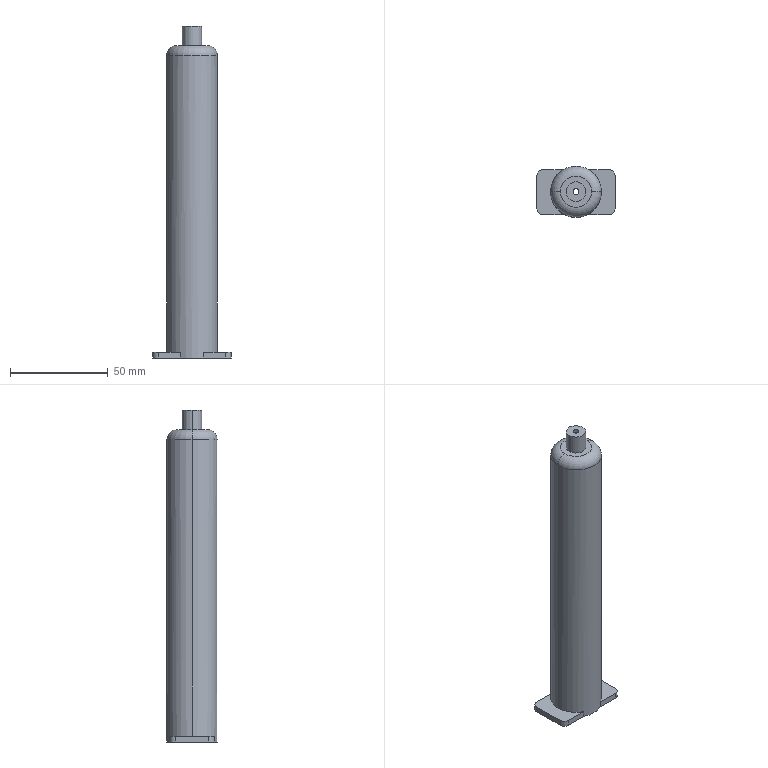Part | NX | features BREP 1 | 1 solid | 31 faces | box 40 x 26 x 170 mm | volume 26319 mm3 | cylinder 14 | plane 13 | torus 4 | commonest cylinder face diameters 6 x6 3 x2 10 x2 22 x2 26 x2
STEP:
#1=CARTESIAN_POINT('',(-1.5,0.,83.));
#2=VERTEX_POINT('',#1);
#3=CARTESIAN_POINT('',(1.5,0.,83.));
#4=VERTEX_POINT('',#3);
#5=CARTESIAN_POINT('',(0.,0.,83.));
#6=DIRECTION('',(0.,0.,1.));
#7=DIRECTION('',(1.,0.,0.));
#8=AXIS2_PLACEMENT_3D('',#5,#6,#7);
#9=CIRCLE('',#8,1.5);
#10=EDGE_CURVE('',#2,#4,#9,.T.);
#11=ORIENTED_EDGE('',*,*,#10,.F.);
#12=CARTESIAN_POINT('',(-1.5,0.,85.));
#13=VERTEX_POINT('',#12);
#14=CARTESIAN_POINT('',(-1.5,0.,75.));
#15=DIRECTION('',(0.,0.,1.));
#16=VECTOR('',#15,1000.);
#17=LINE('',#14,#16);
#18=EDGE_CURVE('',#13,#2,#17,.F.);
#19=ORIENTED_EDGE('',*,*,#18,.F.);
#20=CARTESIAN_POINT('',(1.5,0.,85.));
#21=VERTEX_POINT('',#20);
#22=CARTESIAN_POINT('',(0.,0.,85.));
#23=DIRECTION('',(0.,0.,1.));
#24=DIRECTION('',(1.,0.,0.));
#25=AXIS2_PLACEMENT_3D('',#22,#23,#24);
#26=CIRCLE('',#25,1.5);
#27=EDGE_CURVE('',#13,#21,#26,.T.);
#28=ORIENTED_EDGE('',*,*,#27,.T.);
#29=CARTESIAN_POINT('',(1.5,0.,75.));
#30=DIRECTION('',(0.,0.,1.));
#31=VECTOR('',#30,1000.);
#32=LINE('',#29,#31);
#33=EDGE_CURVE('',#21,#4,#32,.F.);
#34=ORIENTED_EDGE('',*,*,#33,.T.);
#35=EDGE_LOOP('',(#11,#19,#28,#34));
#36=FACE_BOUND('',#35,.T.);
#37=CARTESIAN_POINT('',(0.,0.,75.));
#38=DIRECTION('',(0.,0.,1.));
#39=DIRECTION('',(1.,0.,0.));
#40=AXIS2_PLACEMENT_3D('',#37,#38,#39);
#41=CYLINDRICAL_SURFACE('',#40,1.5);
#42=ADVANCED_FACE('',(#36),#41,.F.);
#43=CARTESIAN_POINT('',(11.,0.,70.));
#44=VERTEX_POINT('',#43);
#45=CARTESIAN_POINT('',(-11.,0.,70.));
#46=VERTEX_POINT('',#45);
#47=CARTESIAN_POINT('',(0.,0.,70.));
#48=DIRECTION('',(0.,0.,-1.));
#49=DIRECTION('',(-1.,0.,0.));
#50=AXIS2_PLACEMENT_3D('',#47,#48,#49);
#51=CIRCLE('',#50,11.);
#52=EDGE_CURVE('',#44,#46,#51,.T.);
#53=ORIENTED_EDGE('',*,*,#52,.T.);
#54=CARTESIAN_POINT('',(-8.,0.,73.));
#55=VERTEX_POINT('',#54);
#56=CARTESIAN_POINT('',(-8.,0.,70.));
#57=DIRECTION('',(0.,1.,0.));
#58=DIRECTION('',(-1.,0.,0.));
#59=AXIS2_PLACEMENT_3D('',#56,#57,#58);
#60=CIRCLE('',#59,3.);
#61=EDGE_CURVE('',#55,#46,#60,.F.);
#62=ORIENTED_EDGE('',*,*,#61,.F.);
#63=CARTESIAN_POINT('',(8.,0.,73.));
#64=VERTEX_POINT('',#63);
#65=CARTESIAN_POINT('',(0.,0.,73.));
#66=DIRECTION('',(0.,0.,1.));
#67=DIRECTION('',(1.,0.,0.));
#68=AXIS2_PLACEMENT_3D('',#65,#66,#67);
#69=CIRCLE('',#68,8.);
#70=EDGE_CURVE('',#55,#64,#69,.T.);
#71=ORIENTED_EDGE('',*,*,#70,.T.);
#72=CARTESIAN_POINT('',(8.,0.,70.));
#73=DIRECTION('',(0.,-1.,0.));
#74=DIRECTION('',(0.,0.,-1.));
#75=AXIS2_PLACEMENT_3D('',#72,#73,#74);
#76=CIRCLE('',#75,3.);
#77=EDGE_CURVE('',#64,#44,#76,.F.);
#78=ORIENTED_EDGE('',*,*,#77,.T.);
#79=EDGE_LOOP('',(#53,#62,#71,#78));
#80=FACE_BOUND('',#79,.T.);
#81=CARTESIAN_POINT('',(0.,0.,70.));
#82=DIRECTION('',(0.,0.,1.));
#83=DIRECTION('',(1.,0.,0.));
#84=AXIS2_PLACEMENT_3D('',#81,#82,#83);
#85=TOROIDAL_SURFACE('',#84,8.,3.);
#86=ADVANCED_FACE('',(#80),#85,.F.);
#87=CARTESIAN_POINT('',(-3.,0.,73.));
#88=VERTEX_POINT('',#87);
#89=CARTESIAN_POINT('',(3.,0.,73.));
#90=VERTEX_POINT('',#89);
#91=CARTESIAN_POINT('',(0.,0.,73.));
#92=DIRECTION('',(0.,0.,1.));
#93=DIRECTION('',(1.,0.,0.));
#94=AXIS2_PLACEMENT_3D('',#91,#92,#93);
#95=CIRCLE('',#94,3.);
#96=EDGE_CURVE('',#88,#90,#95,.T.);
#97=ORIENTED_EDGE('',*,*,#96,.F.);
#98=CARTESIAN_POINT('',(-3.,0.,83.));
#99=VERTEX_POINT('',#98);
#100=CARTESIAN_POINT('',(-3.,0.,75.));
#101=DIRECTION('',(0.,0.,1.));
#102=VECTOR('',#101,1000.);
#103=LINE('',#100,#102);
#104=EDGE_CURVE('',#99,#88,#103,.F.);
#105=ORIENTED_EDGE('',*,*,#104,.F.);
#106=CARTESIAN_POINT('',(3.,0.,83.));
#107=VERTEX_POINT('',#106);
#108=CARTESIAN_POINT('',(0.,0.,83.));
#109=DIRECTION('',(0.,0.,1.));
#110=DIRECTION('',(1.,0.,0.));
#111=AXIS2_PLACEMENT_3D('',#108,#109,#110);
#112=CIRCLE('',#111,3.);
#113=EDGE_CURVE('',#99,#107,#112,.T.);
#114=ORIENTED_EDGE('',*,*,#113,.T.);
#115=CARTESIAN_POINT('',(3.,0.,75.));
#116=DIRECTION('',(0.,0.,1.));
#117=VECTOR('',#116,1000.);
#118=LINE('',#115,#117);
#119=EDGE_CURVE('',#107,#90,#118,.F.);
#120=ORIENTED_EDGE('',*,*,#119,.T.);
#121=EDGE_LOOP('',(#97,#105,#114,#120));
#122=FACE_BOUND('',#121,.T.);
#123=CARTESIAN_POINT('',(0.,0.,75.));
#124=DIRECTION('',(0.,0.,1.));
#125=DIRECTION('',(1.,0.,0.));
#126=AXIS2_PLACEMENT_3D('',#123,#124,#125);
#127=CYLINDRICAL_SURFACE('',#126,3.);
#128=ADVANCED_FACE('',(#122),#127,.F.);
#129=ORIENTED_EDGE('',*,*,#52,.F.);
#130=CARTESIAN_POINT('',(11.,0.,-85.));
#131=VERTEX_POINT('',#130);
#132=CARTESIAN_POINT('',(11.,0.,85.));
#133=DIRECTION('',(0.,0.,-1.));
#134=VECTOR('',#133,1000.);
#135=LINE('',#132,#134);
#136=EDGE_CURVE('',#44,#131,#135,.T.);
#137=ORIENTED_EDGE('',*,*,#136,.T.);
#138=CARTESIAN_POINT('',(-11.,0.,-85.));
#139=VERTEX_POINT('',#138);
#140=CARTESIAN_POINT('',(0.,0.,-85.));
#141=DIRECTION('',(0.,0.,1.));
#142=DIRECTION('',(1.,0.,0.));
#143=AXIS2_PLACEMENT_3D('',#140,#141,#142);
#144=CIRCLE('',#143,11.);
#145=EDGE_CURVE('',#139,#131,#144,.T.);
#146=ORIENTED_EDGE('',*,*,#145,.F.);
#147=CARTESIAN_POINT('',(-11.,0.,85.));
#148=DIRECTION('',(0.,0.,-1.));
#149=VECTOR('',#148,1000.);
#150=LINE('',#147,#149);
#151=EDGE_CURVE('',#46,#139,#150,.T.);
#152=ORIENTED_EDGE('',*,*,#151,.F.);
#153=EDGE_LOOP('',(#129,#137,#146,#152));
#154=FACE_BOUND('',#153,.T.);
#155=CARTESIAN_POINT('',(0.,0.,85.));
#156=DIRECTION('',(0.,0.,-1.));
#157=DIRECTION('',(-1.,0.,0.));
#158=AXIS2_PLACEMENT_3D('',#155,#156,#157);
#159=CYLINDRICAL_SURFACE('',#158,11.);
#160=ADVANCED_FACE('',(#154),#159,.F.);
#161=CARTESIAN_POINT('',(-13.,0.,70.));
#162=VERTEX_POINT('',#161);
#163=CARTESIAN_POINT('',(13.,0.,70.));
#164=VERTEX_POINT('',#163);
#165=CARTESIAN_POINT('',(0.,0.,70.));
#166=DIRECTION('',(0.,0.,-1.));
#167=DIRECTION('',(1.,0.,0.));
#168=AXIS2_PLACEMENT_3D('',#165,#166,#167);
#169=CIRCLE('',#168,13.);
#170=EDGE_CURVE('',#162,#164,#169,.T.);
#171=ORIENTED_EDGE('',*,*,#170,.F.);
#172=CARTESIAN_POINT('',(-8.,0.,75.));
#173=VERTEX_POINT('',#172);
#174=CARTESIAN_POINT('',(-8.,0.,70.));
#175=DIRECTION('',(0.,1.,0.));
#176=DIRECTION('',(-1.,0.,0.));
#177=AXIS2_PLACEMENT_3D('',#174,#175,#176);
#178=CIRCLE('',#177,5.);
#179=EDGE_CURVE('',#173,#162,#178,.F.);
#180=ORIENTED_EDGE('',*,*,#179,.F.);
#181=CARTESIAN_POINT('',(8.,0.,75.));
#182=VERTEX_POINT('',#181);
#183=CARTESIAN_POINT('',(0.,0.,75.));
#184=DIRECTION('',(0.,0.,1.));
#185=DIRECTION('',(1.,0.,0.));
#186=AXIS2_PLACEMENT_3D('',#183,#184,#185);
#187=CIRCLE('',#186,8.);
#188=EDGE_CURVE('',#182,#173,#187,.T.);
#189=ORIENTED_EDGE('',*,*,#188,.F.);
#190=CARTESIAN_POINT('',(8.,0.,70.));
#191=DIRECTION('',(0.,-1.,0.));
#192=DIRECTION('',(0.,0.,-1.));
#193=AXIS2_PLACEMENT_3D('',#190,#191,#192);
#194=CIRCLE('',#193,5.);
#195=EDGE_CURVE('',#182,#164,#194,.F.);
#196=ORIENTED_EDGE('',*,*,#195,.T.);
#197=EDGE_LOOP('',(#171,#180,#189,#196));
#198=FACE_BOUND('',#197,.T.);
#199=CARTESIAN_POINT('',(0.,0.,70.));
#200=DIRECTION('',(0.,0.,1.));
#201=DIRECTION('',(1.,0.,0.));
#202=AXIS2_PLACEMENT_3D('',#199,#200,#201);
#203=TOROIDAL_SURFACE('',#202,8.,5.);
#204=ADVANCED_FACE('',(#198),#203,.T.);
#205=CARTESIAN_POINT('',(5.,0.,75.));
#206=VERTEX_POINT('',#205);
#207=CARTESIAN_POINT('',(-5.,0.,75.));
#208=VERTEX_POINT('',#207);
#209=CARTESIAN_POINT('',(0.,0.,75.));
#210=DIRECTION('',(0.,0.,1.));
#211=DIRECTION('',(1.,0.,0.));
#212=AXIS2_PLACEMENT_3D('',#209,#210,#211);
#213=CIRCLE('',#212,5.);
#214=EDGE_CURVE('',#206,#208,#213,.T.);
#215=ORIENTED_EDGE('',*,*,#214,.T.);
#216=CARTESIAN_POINT('',(-5.,0.,85.));
#217=VERTEX_POINT('',#216);
#218=CARTESIAN_POINT('',(-5.,0.,75.));
#219=DIRECTION('',(0.,0.,1.));
#220=VECTOR('',#219,1000.);
#221=LINE('',#218,#220);
#222=EDGE_CURVE('',#217,#208,#221,.F.);
#223=ORIENTED_EDGE('',*,*,#222,.F.);
#224=CARTESIAN_POINT('',(5.,0.,85.));
#225=VERTEX_POINT('',#224);
#226=CARTESIAN_POINT('',(0.,0.,85.));
#227=DIRECTION('',(0.,0.,1.));
#228=DIRECTION('',(1.,0.,0.));
#229=AXIS2_PLACEMENT_3D('',#226,#227,#228);
#230=CIRCLE('',#229,5.);
#231=EDGE_CURVE('',#225,#217,#230,.T.);
#232=ORIENTED_EDGE('',*,*,#231,.F.);
#233=CARTESIAN_POINT('',(5.,0.,75.));
#234=DIRECTION('',(0.,0.,1.));
#235=VECTOR('',#234,1000.);
#236=LINE('',#233,#235);
#237=EDGE_CURVE('',#225,#206,#236,.F.);
#238=ORIENTED_EDGE('',*,*,#237,.T.);
#239=EDGE_LOOP('',(#215,#223,#232,#238));
#240=FACE_BOUND('',#239,.T.);
#241=CARTESIAN_POINT('',(0.,0.,75.));
#242=DIRECTION('',(0.,0.,1.));
#243=DIRECTION('',(1.,0.,0.));
#244=AXIS2_PLACEMENT_3D('',#241,#242,#243);
#245=CYLINDRICAL_SURFACE('',#244,5.);
#246=ADVANCED_FACE('',(#240),#245,.T.);
#247=ORIENTED_EDGE('',*,*,#170,.T.);
#248=CARTESIAN_POINT('',(13.,0.,-82.));
#249=VERTEX_POINT('',#248);
#250=CARTESIAN_POINT('',(13.,0.,85.));
#251=DIRECTION('',(0.,0.,-1.));
#252=VECTOR('',#251,1000.);
#253=LINE('',#250,#252);
#254=EDGE_CURVE('',#164,#249,#253,.T.);
#255=ORIENTED_EDGE('',*,*,#254,.T.);
#256=CARTESIAN_POINT('',(6.062,11.5,-82.));
#257=VERTEX_POINT('',#256);
#258=CARTESIAN_POINT('',(0.,0.,-82.));
#259=DIRECTION('',(0.,0.,1.));
#260=DIRECTION('',(-1.,0.,0.));
#261=AXIS2_PLACEMENT_3D('',#258,#259,#260);
#262=CIRCLE('',#261,13.);
#263=EDGE_CURVE('',#249,#257,#262,.T.);
#264=ORIENTED_EDGE('',*,*,#263,.T.);
#265=CARTESIAN_POINT('',(6.062,11.5,-85.));
#266=VERTEX_POINT('',#265);
#267=CARTESIAN_POINT('',(6.062,11.5,-82.));
#268=DIRECTION('',(0.,0.,-1.));
#269=VECTOR('',#268,1000.);
#270=LINE('',#267,#269);
#271=EDGE_CURVE('',#257,#266,#270,.T.);
#272=ORIENTED_EDGE('',*,*,#271,.T.);
#273=CARTESIAN_POINT('',(-6.062,11.5,-85.));
#274=VERTEX_POINT('',#273);
#275=CARTESIAN_POINT('',(0.,0.,-85.));
#276=DIRECTION('',(0.,0.,1.));
#277=DIRECTION('',(1.,0.,0.));
#278=AXIS2_PLACEMENT_3D('',#275,#276,#277);
#279=CIRCLE('',#278,13.);
#280=EDGE_CURVE('',#266,#274,#279,.T.);
#281=ORIENTED_EDGE('',*,*,#280,.T.);
#282=CARTESIAN_POINT('',(-6.062,11.5,-82.));
#283=VERTEX_POINT('',#282);
#284=CARTESIAN_POINT('',(-6.062,11.5,-82.));
#285=DIRECTION('',(0.,0.,-1.));
#286=VECTOR('',#285,1000.);
#287=LINE('',#284,#286);
#288=EDGE_CURVE('',#283,#274,#287,.T.);
#289=ORIENTED_EDGE('',*,*,#288,.F.);
#290=CARTESIAN_POINT('',(-13.,0.,-82.));
#291=VERTEX_POINT('',#290);
#292=CARTESIAN_POINT('',(0.,0.,-82.));
#293=DIRECTION('',(0.,0.,1.));
#294=DIRECTION('',(-1.,0.,0.));
#295=AXIS2_PLACEMENT_3D('',#292,#293,#294);
#296=CIRCLE('',#295,13.);
#297=EDGE_CURVE('',#283,#291,#296,.T.);
#298=ORIENTED_EDGE('',*,*,#297,.T.);
#299=CARTESIAN_POINT('',(-13.,0.,85.));
#300=DIRECTION('',(0.,0.,-1.));
#301=VECTOR('',#300,1000.);
#302=LINE('',#299,#301);
#303=EDGE_CURVE('',#162,#291,#302,.T.);
#304=ORIENTED_EDGE('',*,*,#303,.F.);
#305=EDGE_LOOP('',(#247,#255,#264,#272,#281,#289,#298,#304));
#306=FACE_BOUND('',#305,.T.);
#307=CARTESIAN_POINT('',(0.,0.,85.));
#308=DIRECTION('',(0.,0.,-1.));
#309=DIRECTION('',(-1.,0.,0.));
#310=AXIS2_PLACEMENT_3D('',#307,#308,#309);
#311=CYLINDRICAL_SURFACE('',#310,13.);
#312=ADVANCED_FACE('',(#306),#311,.T.);
#313=ORIENTED_EDGE('',*,*,#254,.F.);
#314=CARTESIAN_POINT('',(0.,0.,70.));
#315=DIRECTION('',(0.,0.,-1.));
#316=DIRECTION('',(1.,0.,0.));
#317=AXIS2_PLACEMENT_3D('',#314,#315,#316);
#318=CIRCLE('',#317,13.);
#319=EDGE_CURVE('',#164,#162,#318,.T.);
#320=ORIENTED_EDGE('',*,*,#319,.T.);
#321=ORIENTED_EDGE('',*,*,#303,.T.);
#322=CARTESIAN_POINT('',(-6.062,-11.5,-82.));
#323=VERTEX_POINT('',#322);
#324=CARTESIAN_POINT('',(0.,0.,-82.));
#325=DIRECTION('',(0.,0.,1.));
#326=DIRECTION('',(-1.,0.,0.));
#327=AXIS2_PLACEMENT_3D('',#324,#325,#326);
#328=CIRCLE('',#327,13.);
#329=EDGE_CURVE('',#291,#323,#328,.T.);
#330=ORIENTED_EDGE('',*,*,#329,.T.);
#331=CARTESIAN_POINT('',(-6.062,-11.5,-85.));
#332=VERTEX_POINT('',#331);
#333=CARTESIAN_POINT('',(-6.062,-11.5,-82.));
#334=DIRECTION('',(0.,0.,-1.));
#335=VECTOR('',#334,1000.);
#336=LINE('',#333,#335);
#337=EDGE_CURVE('',#323,#332,#336,.T.);
#338=ORIENTED_EDGE('',*,*,#337,.T.);
#339=CARTESIAN_POINT('',(6.062,-11.5,-85.));
#340=VERTEX_POINT('',#339);
#341=CARTESIAN_POINT('',(0.,0.,-85.));
#342=DIRECTION('',(0.,0.,1.));
#343=DIRECTION('',(1.,0.,0.));
#344=AXIS2_PLACEMENT_3D('',#341,#342,#343);
#345=CIRCLE('',#344,13.);
#346=EDGE_CURVE('',#332,#340,#345,.T.);
#347=ORIENTED_EDGE('',*,*,#346,.T.);
#348=CARTESIAN_POINT('',(6.062,-11.5,-82.));
#349=VERTEX_POINT('',#348);
#350=CARTESIAN_POINT('',(6.062,-11.5,-82.));
#351=DIRECTION('',(0.,0.,-1.));
#352=VECTOR('',#351,1000.);
#353=LINE('',#350,#352);
#354=EDGE_CURVE('',#349,#340,#353,.T.);
#355=ORIENTED_EDGE('',*,*,#354,.F.);
#356=CARTESIAN_POINT('',(0.,0.,-82.));
#357=DIRECTION('',(0.,0.,1.));
#358=DIRECTION('',(-1.,0.,0.));
#359=AXIS2_PLACEMENT_3D('',#356,#357,#358);
#360=CIRCLE('',#359,13.);
#361=EDGE_CURVE('',#349,#249,#360,.T.);
#362=ORIENTED_EDGE('',*,*,#361,.T.);
#363=EDGE_LOOP('',(#313,#320,#321,#330,#338,#347,#355,#362));
#364=FACE_BOUND('',#363,.T.);
#365=CARTESIAN_POINT('',(0.,0.,85.));
#366=DIRECTION('',(0.,0.,-1.));
#367=DIRECTION('',(-1.,0.,0.));
#368=AXIS2_PLACEMENT_3D('',#365,#366,#367);
#369=CYLINDRICAL_SURFACE('',#368,13.);
#370=ADVANCED_FACE('',(#364),#369,.T.);
#371=CARTESIAN_POINT('',(-20.,-8.5,-85.));
#372=VERTEX_POINT('',#371);
#373=CARTESIAN_POINT('',(-20.,8.5,-85.));
#374=VERTEX_POINT('',#373);
#375=CARTESIAN_POINT('',(-20.,11.5,-85.));
#376=DIRECTION('',(0.,1.,0.));
#377=VECTOR('',#376,1000.);
#378=LINE('',#375,#377);
#379=EDGE_CURVE('',#372,#374,#378,.T.);
#380=ORIENTED_EDGE('',*,*,#379,.T.);
#381=CARTESIAN_POINT('',(-17.,11.5,-85.));
#382=VERTEX_POINT('',#381);
#383=CARTESIAN_POINT('',(-17.,8.5,-85.));
#384=DIRECTION('',(0.,0.,-1.));
#385=DIRECTION('',(1.,0.,0.));
#386=AXIS2_PLACEMENT_3D('',#383,#384,#385);
#387=CIRCLE('',#386,3.);
#388=EDGE_CURVE('',#374,#382,#387,.T.);
#389=ORIENTED_EDGE('',*,*,#388,.T.);
#390=CARTESIAN_POINT('',(-6.062,11.5,-85.));
#391=DIRECTION('',(1.,0.,0.));
#392=VECTOR('',#391,1000.);
#393=LINE('',#390,#392);
#394=EDGE_CURVE('',#382,#274,#393,.T.);
#395=ORIENTED_EDGE('',*,*,#394,.T.);
#396=ORIENTED_EDGE('',*,*,#280,.F.);
#397=CARTESIAN_POINT('',(17.,11.5,-85.));
#398=VERTEX_POINT('',#397);
#399=CARTESIAN_POINT('',(6.062,11.5,-85.));
#400=DIRECTION('',(1.,0.,0.));
#401=VECTOR('',#400,1000.);
#402=LINE('',#399,#401);
#403=EDGE_CURVE('',#266,#398,#402,.T.);
#404=ORIENTED_EDGE('',*,*,#403,.T.);
#405=CARTESIAN_POINT('',(20.,8.5,-85.));
#406=VERTEX_POINT('',#405);
#407=CARTESIAN_POINT('',(17.,8.5,-85.));
#408=DIRECTION('',(0.,0.,-1.));
#409=DIRECTION('',(1.,0.,0.));
#410=AXIS2_PLACEMENT_3D('',#407,#408,#409);
#411=CIRCLE('',#410,3.);
#412=EDGE_CURVE('',#398,#406,#411,.T.);
#413=ORIENTED_EDGE('',*,*,#412,.T.);
#414=CARTESIAN_POINT('',(20.,-8.5,-85.));
#415=VERTEX_POINT('',#414);
#416=CARTESIAN_POINT('',(20.,11.5,-85.));
#417=DIRECTION('',(0.,-1.,0.));
#418=VECTOR('',#417,1000.);
#419=LINE('',#416,#418);
#420=EDGE_CURVE('',#406,#415,#419,.T.);
#421=ORIENTED_EDGE('',*,*,#420,.T.);
#422=CARTESIAN_POINT('',(17.,-11.5,-85.));
#423=VERTEX_POINT('',#422);
#424=CARTESIAN_POINT('',(17.,-8.5,-85.));
#425=DIRECTION('',(0.,0.,-1.));
#426=DIRECTION('',(1.,0.,0.));
#427=AXIS2_PLACEMENT_3D('',#424,#425,#426);
#428=CIRCLE('',#427,3.);
#429=EDGE_CURVE('',#415,#423,#428,.T.);
#430=ORIENTED_EDGE('',*,*,#429,.T.);
#431=CARTESIAN_POINT('',(20.,-11.5,-85.));
#432=DIRECTION('',(-1.,0.,0.));
#433=VECTOR('',#432,1000.);
#434=LINE('',#431,#433);
#435=EDGE_CURVE('',#423,#340,#434,.T.);
#436=ORIENTED_EDGE('',*,*,#435,.T.);
#437=ORIENTED_EDGE('',*,*,#346,.F.);
#438=CARTESIAN_POINT('',(-17.,-11.5,-85.));
#439=VERTEX_POINT('',#438);
#440=CARTESIAN_POINT('',(-20.,-11.5,-85.));
#441=DIRECTION('',(-1.,0.,0.));
#442=VECTOR('',#441,1000.);
#443=LINE('',#440,#442);
#444=EDGE_CURVE('',#332,#439,#443,.T.);
#445=ORIENTED_EDGE('',*,*,#444,.T.);
#446=CARTESIAN_POINT('',(-17.,-8.5,-85.));
#447=DIRECTION('',(0.,0.,-1.));
#448=DIRECTION('',(1.,0.,0.));
#449=AXIS2_PLACEMENT_3D('',#446,#447,#448);
#450=CIRCLE('',#449,3.);
#451=EDGE_CURVE('',#439,#372,#450,.T.);
#452=ORIENTED_EDGE('',*,*,#451,.T.);
#453=EDGE_LOOP('',(#380,#389,#395,#396,#404,#413,#421,#430,#436,#437,#445,#452));
#454=FACE_BOUND('',#453,.T.);
#455=ORIENTED_EDGE('',*,*,#145,.T.);
#456=CARTESIAN_POINT('',(0.,0.,-85.));
#457=DIRECTION('',(0.,0.,1.));
#458=DIRECTION('',(1.,0.,0.));
#459=AXIS2_PLACEMENT_3D('',#456,#457,#458);
#460=CIRCLE('',#459,11.);
#461=EDGE_CURVE('',#131,#139,#460,.T.);
#462=ORIENTED_EDGE('',*,*,#461,.T.);
#463=EDGE_LOOP('',(#455,#462));
#464=FACE_BOUND('',#463,.T.);
#465=CARTESIAN_POINT('',(0.,0.,-85.));
#466=DIRECTION('',(0.,0.,1.));
#467=DIRECTION('',(1.,0.,0.));
#468=AXIS2_PLACEMENT_3D('',#465,#466,#467);
#469=PLANE('',#468);
#470=ADVANCED_FACE('',(#454,#464),#469,.F.);
#471=ORIENTED_EDGE('',*,*,#188,.T.);
#472=CARTESIAN_POINT('',(0.,0.,75.));
#473=DIRECTION('',(0.,0.,1.));
#474=DIRECTION('',(1.,0.,0.));
#475=AXIS2_PLACEMENT_3D('',#472,#473,#474);
#476=CIRCLE('',#475,8.);
#477=EDGE_CURVE('',#173,#182,#476,.T.);
#478=ORIENTED_EDGE('',*,*,#477,.T.);
#479=EDGE_LOOP('',(#471,#478));
#480=FACE_BOUND('',#479,.T.);
#481=ORIENTED_EDGE('',*,*,#214,.F.);
#482=CARTESIAN_POINT('',(0.,0.,75.));
#483=DIRECTION('',(0.,0.,1.));
#484=DIRECTION('',(1.,0.,0.));
#485=AXIS2_PLACEMENT_3D('',#482,#483,#484);
#486=CIRCLE('',#485,5.);
#487=EDGE_CURVE('',#208,#206,#486,.T.);
#488=ORIENTED_EDGE('',*,*,#487,.F.);
#489=EDGE_LOOP('',(#481,#488));
#490=FACE_BOUND('',#489,.T.);
#491=CARTESIAN_POINT('',(0.,0.,75.));
#492=DIRECTION('',(0.,0.,1.));
#493=DIRECTION('',(1.,0.,0.));
#494=AXIS2_PLACEMENT_3D('',#491,#492,#493);
#495=PLANE('',#494);
#496=ADVANCED_FACE('',(#480,#490),#495,.T.);
#497=ORIENTED_EDGE('',*,*,#222,.T.);
#498=ORIENTED_EDGE('',*,*,#487,.T.);
#499=ORIENTED_EDGE('',*,*,#237,.F.);
#500=CARTESIAN_POINT('',(0.,0.,85.));
#501=DIRECTION('',(0.,0.,1.));
#502=DIRECTION('',(1.,0.,0.));
#503=AXIS2_PLACEMENT_3D('',#500,#501,#502);
#504=CIRCLE('',#503,5.);
#505=EDGE_CURVE('',#217,#225,#504,.T.);
#506=ORIENTED_EDGE('',*,*,#505,.F.);
#507=EDGE_LOOP('',(#497,#498,#499,#506));
#508=FACE_BOUND('',#507,.T.);
#509=CARTESIAN_POINT('',(0.,0.,75.));
#510=DIRECTION('',(0.,0.,1.));
#511=DIRECTION('',(1.,0.,0.));
#512=AXIS2_PLACEMENT_3D('',#509,#510,#511);
#513=CYLINDRICAL_SURFACE('',#512,5.);
#514=ADVANCED_FACE('',(#508),#513,.T.);
#515=ORIENTED_EDGE('',*,*,#231,.T.);
#516=ORIENTED_EDGE('',*,*,#505,.T.);
#517=EDGE_LOOP('',(#515,#516));
#518=FACE_BOUND('',#517,.T.);
#519=CARTESIAN_POINT('',(0.,0.,85.));
#520=DIRECTION('',(0.,0.,1.));
#521=DIRECTION('',(1.,0.,0.));
#522=AXIS2_PLACEMENT_3D('',#519,#520,#521);
#523=CIRCLE('',#522,1.5);
#524=EDGE_CURVE('',#21,#13,#523,.T.);
#525=ORIENTED_EDGE('',*,*,#524,.F.);
#526=ORIENTED_EDGE('',*,*,#27,.F.);
#527=EDGE_LOOP('',(#525,#526));
#528=FACE_BOUND('',#527,.T.);
#529=CARTESIAN_POINT('',(0.,0.,85.));
#530=DIRECTION('',(0.,0.,1.));
#531=DIRECTION('',(1.,0.,0.));
#532=AXIS2_PLACEMENT_3D('',#529,#530,#531);
#533=PLANE('',#532);
#534=ADVANCED_FACE('',(#518,#528),#533,.T.);
#535=ORIENTED_EDGE('',*,*,#179,.T.);
#536=ORIENTED_EDGE('',*,*,#319,.F.);
#537=ORIENTED_EDGE('',*,*,#195,.F.);
#538=ORIENTED_EDGE('',*,*,#477,.F.);
#539=EDGE_LOOP('',(#535,#536,#537,#538));
#540=FACE_BOUND('',#539,.T.);
#541=CARTESIAN_POINT('',(0.,0.,70.));
#542=DIRECTION('',(0.,0.,1.));
#543=DIRECTION('',(1.,0.,0.));
#544=AXIS2_PLACEMENT_3D('',#541,#542,#543);
#545=TOROIDAL_SURFACE('',#544,8.,5.);
#546=ADVANCED_FACE('',(#540),#545,.T.);
#547=ORIENTED_EDGE('',*,*,#136,.F.);
#548=CARTESIAN_POINT('',(0.,0.,70.));
#549=DIRECTION('',(0.,0.,-1.));
#550=DIRECTION('',(-1.,0.,0.));
#551=AXIS2_PLACEMENT_3D('',#548,#549,#550);
#552=CIRCLE('',#551,11.);
#553=EDGE_CURVE('',#46,#44,#552,.T.);
#554=ORIENTED_EDGE('',*,*,#553,.F.);
#555=ORIENTED_EDGE('',*,*,#151,.T.);
#556=ORIENTED_EDGE('',*,*,#461,.F.);
#557=EDGE_LOOP('',(#547,#554,#555,#556));
#558=FACE_BOUND('',#557,.T.);
#559=CARTESIAN_POINT('',(0.,0.,85.));
#560=DIRECTION('',(0.,0.,-1.));
#561=DIRECTION('',(-1.,0.,0.));
#562=AXIS2_PLACEMENT_3D('',#559,#560,#561);
#563=CYLINDRICAL_SURFACE('',#562,11.);
#564=ADVANCED_FACE('',(#558),#563,.F.);
#565=CARTESIAN_POINT('',(0.,0.,73.));
#566=DIRECTION('',(0.,0.,1.));
#567=DIRECTION('',(1.,0.,0.));
#568=AXIS2_PLACEMENT_3D('',#565,#566,#567);
#569=CIRCLE('',#568,8.);
#570=EDGE_CURVE('',#64,#55,#569,.T.);
#571=ORIENTED_EDGE('',*,*,#570,.F.);
#572=ORIENTED_EDGE('',*,*,#70,.F.);
#573=EDGE_LOOP('',(#571,#572));
#574=FACE_BOUND('',#573,.T.);
#575=CARTESIAN_POINT('',(0.,0.,73.));
#576=DIRECTION('',(0.,0.,1.));
#577=DIRECTION('',(1.,0.,0.));
#578=AXIS2_PLACEMENT_3D('',#575,#576,#577);
#579=CIRCLE('',#578,3.);
#580=EDGE_CURVE('',#90,#88,#579,.T.);
#581=ORIENTED_EDGE('',*,*,#580,.T.);
#582=ORIENTED_EDGE('',*,*,#96,.T.);
#583=EDGE_LOOP('',(#581,#582));
#584=FACE_BOUND('',#583,.T.);
#585=CARTESIAN_POINT('',(0.,0.,73.));
#586=DIRECTION('',(0.,0.,1.));
#587=DIRECTION('',(1.,0.,0.));
#588=AXIS2_PLACEMENT_3D('',#585,#586,#587);
#589=PLANE('',#588);
#590=ADVANCED_FACE('',(#574,#584),#589,.F.);
#591=ORIENTED_EDGE('',*,*,#104,.T.);
#592=ORIENTED_EDGE('',*,*,#580,.F.);
#593=ORIENTED_EDGE('',*,*,#119,.F.);
#594=CARTESIAN_POINT('',(0.,0.,83.));
#595=DIRECTION('',(0.,0.,1.));
#596=DIRECTION('',(1.,0.,0.));
#597=AXIS2_PLACEMENT_3D('',#594,#595,#596);
#598=CIRCLE('',#597,3.);
#599=EDGE_CURVE('',#107,#99,#598,.T.);
#600=ORIENTED_EDGE('',*,*,#599,.T.);
#601=EDGE_LOOP('',(#591,#592,#593,#600));
#602=FACE_BOUND('',#601,.T.);
#603=CARTESIAN_POINT('',(0.,0.,75.));
#604=DIRECTION('',(0.,0.,1.));
#605=DIRECTION('',(1.,0.,0.));
#606=AXIS2_PLACEMENT_3D('',#603,#604,#605);
#607=CYLINDRICAL_SURFACE('',#606,3.);
#608=ADVANCED_FACE('',(#602),#607,.F.);
#609=ORIENTED_EDGE('',*,*,#599,.F.);
#610=ORIENTED_EDGE('',*,*,#113,.F.);
#611=EDGE_LOOP('',(#609,#610));
#612=FACE_BOUND('',#611,.T.);
#613=CARTESIAN_POINT('',(0.,0.,83.));
#614=DIRECTION('',(0.,0.,1.));
#615=DIRECTION('',(1.,0.,0.));
#616=AXIS2_PLACEMENT_3D('',#613,#614,#615);
#617=CIRCLE('',#616,1.5);
#618=EDGE_CURVE('',#4,#2,#617,.T.);
#619=ORIENTED_EDGE('',*,*,#618,.T.);
#620=ORIENTED_EDGE('',*,*,#10,.T.);
#621=EDGE_LOOP('',(#619,#620));
#622=FACE_BOUND('',#621,.T.);
#623=CARTESIAN_POINT('',(0.,0.,83.));
#624=DIRECTION('',(0.,0.,1.));
#625=DIRECTION('',(1.,0.,0.));
#626=AXIS2_PLACEMENT_3D('',#623,#624,#625);
#627=PLANE('',#626);
#628=ADVANCED_FACE('',(#612,#622),#627,.F.);
#629=ORIENTED_EDGE('',*,*,#61,.T.);
#630=ORIENTED_EDGE('',*,*,#553,.T.);
#631=ORIENTED_EDGE('',*,*,#77,.F.);
#632=ORIENTED_EDGE('',*,*,#570,.T.);
#633=EDGE_LOOP('',(#629,#630,#631,#632));
#634=FACE_BOUND('',#633,.T.);
#635=CARTESIAN_POINT('',(0.,0.,70.));
#636=DIRECTION('',(0.,0.,1.));
#637=DIRECTION('',(1.,0.,0.));
#638=AXIS2_PLACEMENT_3D('',#635,#636,#637);
#639=TOROIDAL_SURFACE('',#638,8.,3.);
#640=ADVANCED_FACE('',(#634),#639,.F.);
#641=ORIENTED_EDGE('',*,*,#18,.T.);
#642=ORIENTED_EDGE('',*,*,#618,.F.);
#643=ORIENTED_EDGE('',*,*,#33,.F.);
#644=ORIENTED_EDGE('',*,*,#524,.T.);
#645=EDGE_LOOP('',(#641,#642,#643,#644));
#646=FACE_BOUND('',#645,.T.);
#647=CARTESIAN_POINT('',(0.,0.,75.));
#648=DIRECTION('',(0.,0.,1.));
#649=DIRECTION('',(1.,0.,0.));
#650=AXIS2_PLACEMENT_3D('',#647,#648,#649);
#651=CYLINDRICAL_SURFACE('',#650,1.5);
#652=ADVANCED_FACE('',(#646),#651,.F.);
#653=CARTESIAN_POINT('',(-20.,-8.5,-82.));
#654=VERTEX_POINT('',#653);
#655=CARTESIAN_POINT('',(-20.,8.5,-82.));
#656=VERTEX_POINT('',#655);
#657=CARTESIAN_POINT('',(-20.,11.5,-82.));
#658=DIRECTION('',(0.,1.,0.));
#659=VECTOR('',#658,1000.);
#660=LINE('',#657,#659);
#661=EDGE_CURVE('',#654,#656,#660,.T.);
#662=ORIENTED_EDGE('',*,*,#661,.T.);
#663=CARTESIAN_POINT('',(-20.,8.5,-82.));
#664=DIRECTION('',(0.,0.,-1.));
#665=VECTOR('',#664,1000.);
#666=LINE('',#663,#665);
#667=EDGE_CURVE('',#656,#374,#666,.T.);
#668=ORIENTED_EDGE('',*,*,#667,.T.);
#669=ORIENTED_EDGE('',*,*,#379,.F.);
#670=CARTESIAN_POINT('',(-20.,-8.5,-82.));
#671=DIRECTION('',(0.,0.,1.));
#672=VECTOR('',#671,1000.);
#673=LINE('',#670,#672);
#674=EDGE_CURVE('',#372,#654,#673,.T.);
#675=ORIENTED_EDGE('',*,*,#674,.T.);
#676=EDGE_LOOP('',(#662,#668,#669,#675));
#677=FACE_BOUND('',#676,.T.);
#678=CARTESIAN_POINT('',(-20.,11.5,-82.));
#679=DIRECTION('',(-1.,0.,0.));
#680=DIRECTION('',(0.,0.,1.));
#681=AXIS2_PLACEMENT_3D('',#678,#679,#680);
#682=PLANE('',#681);
#683=ADVANCED_FACE('',(#677),#682,.T.);
#684=CARTESIAN_POINT('',(-17.,-11.5,-82.));
#685=VERTEX_POINT('',#684);
#686=CARTESIAN_POINT('',(-20.,-11.5,-82.));
#687=DIRECTION('',(-1.,0.,0.));
#688=VECTOR('',#687,1000.);
#689=LINE('',#686,#688);
#690=EDGE_CURVE('',#323,#685,#689,.T.);
#691=ORIENTED_EDGE('',*,*,#690,.T.);
#692=CARTESIAN_POINT('',(-17.,-11.5,-82.));
#693=DIRECTION('',(0.,0.,-1.));
#694=VECTOR('',#693,1000.);
#695=LINE('',#692,#694);
#696=EDGE_CURVE('',#685,#439,#695,.T.);
#697=ORIENTED_EDGE('',*,*,#696,.T.);
#698=ORIENTED_EDGE('',*,*,#444,.F.);
#699=ORIENTED_EDGE('',*,*,#337,.F.);
#700=EDGE_LOOP('',(#691,#697,#698,#699));
#701=FACE_BOUND('',#700,.T.);
#702=CARTESIAN_POINT('',(-20.,-11.5,-82.));
#703=DIRECTION('',(0.,-1.,0.));
#704=DIRECTION('',(0.,0.,-1.));
#705=AXIS2_PLACEMENT_3D('',#702,#703,#704);
#706=PLANE('',#705);
#707=ADVANCED_FACE('',(#701),#706,.T.);
#708=ORIENTED_EDGE('',*,*,#394,.F.);
#709=CARTESIAN_POINT('',(-17.,11.5,-82.));
#710=VERTEX_POINT('',#709);
#711=CARTESIAN_POINT('',(-17.,11.5,-82.));
#712=DIRECTION('',(0.,0.,1.));
#713=VECTOR('',#712,1000.);
#714=LINE('',#711,#713);
#715=EDGE_CURVE('',#382,#710,#714,.T.);
#716=ORIENTED_EDGE('',*,*,#715,.T.);
#717=CARTESIAN_POINT('',(-6.062,11.5,-82.));
#718=DIRECTION('',(1.,0.,0.));
#719=VECTOR('',#718,1000.);
#720=LINE('',#717,#719);
#721=EDGE_CURVE('',#710,#283,#720,.T.);
#722=ORIENTED_EDGE('',*,*,#721,.T.);
#723=ORIENTED_EDGE('',*,*,#288,.T.);
#724=EDGE_LOOP('',(#708,#716,#722,#723));
#725=FACE_BOUND('',#724,.T.);
#726=CARTESIAN_POINT('',(-6.062,11.5,-82.));
#727=DIRECTION('',(0.,1.,0.));
#728=DIRECTION('',(1.,0.,0.));
#729=AXIS2_PLACEMENT_3D('',#726,#727,#728);
#730=PLANE('',#729);
#731=ADVANCED_FACE('',(#725),#730,.T.);
#732=ORIENTED_EDGE('',*,*,#721,.F.);
#733=CARTESIAN_POINT('',(-17.,8.5,-82.));
#734=DIRECTION('',(0.,0.,1.));
#735=DIRECTION('',(-1.,0.,0.));
#736=AXIS2_PLACEMENT_3D('',#733,#734,#735);
#737=CIRCLE('',#736,3.);
#738=EDGE_CURVE('',#710,#656,#737,.T.);
#739=ORIENTED_EDGE('',*,*,#738,.T.);
#740=ORIENTED_EDGE('',*,*,#661,.F.);
#741=CARTESIAN_POINT('',(-17.,-8.5,-82.));
#742=DIRECTION('',(0.,0.,1.));
#743=DIRECTION('',(-1.,0.,0.));
#744=AXIS2_PLACEMENT_3D('',#741,#742,#743);
#745=CIRCLE('',#744,3.);
#746=EDGE_CURVE('',#654,#685,#745,.T.);
#747=ORIENTED_EDGE('',*,*,#746,.T.);
#748=ORIENTED_EDGE('',*,*,#690,.F.);
#749=ORIENTED_EDGE('',*,*,#329,.F.);
#750=ORIENTED_EDGE('',*,*,#297,.F.);
#751=EDGE_LOOP('',(#732,#739,#740,#747,#748,#749,#750));
#752=FACE_BOUND('',#751,.T.);
#753=CARTESIAN_POINT('',(0.,0.,-82.));
#754=DIRECTION('',(0.,0.,-1.));
#755=DIRECTION('',(0.,-1.,0.));
#756=AXIS2_PLACEMENT_3D('',#753,#754,#755);
#757=PLANE('',#756);
#758=ADVANCED_FACE('',(#752),#757,.F.);
#759=ORIENTED_EDGE('',*,*,#420,.F.);
#760=CARTESIAN_POINT('',(20.,8.5,-82.));
#761=VERTEX_POINT('',#760);
#762=CARTESIAN_POINT('',(20.,8.5,-82.));
#763=DIRECTION('',(0.,0.,1.));
#764=VECTOR('',#763,1000.);
#765=LINE('',#762,#764);
#766=EDGE_CURVE('',#406,#761,#765,.T.);
#767=ORIENTED_EDGE('',*,*,#766,.T.);
#768=CARTESIAN_POINT('',(20.,-8.5,-82.));
#769=VERTEX_POINT('',#768);
#770=CARTESIAN_POINT('',(20.,11.5,-82.));
#771=DIRECTION('',(0.,-1.,0.));
#772=VECTOR('',#771,1000.);
#773=LINE('',#770,#772);
#774=EDGE_CURVE('',#761,#769,#773,.T.);
#775=ORIENTED_EDGE('',*,*,#774,.T.);
#776=CARTESIAN_POINT('',(20.,-8.5,-82.));
#777=DIRECTION('',(0.,0.,-1.));
#778=VECTOR('',#777,1000.);
#779=LINE('',#776,#778);
#780=EDGE_CURVE('',#769,#415,#779,.T.);
#781=ORIENTED_EDGE('',*,*,#780,.T.);
#782=EDGE_LOOP('',(#759,#767,#775,#781));
#783=FACE_BOUND('',#782,.T.);
#784=CARTESIAN_POINT('',(20.,11.5,-82.));
#785=DIRECTION('',(1.,0.,0.));
#786=DIRECTION('',(0.,1.,0.));
#787=AXIS2_PLACEMENT_3D('',#784,#785,#786);
#788=PLANE('',#787);
#789=ADVANCED_FACE('',(#783),#788,.T.);
#790=CARTESIAN_POINT('',(17.,11.5,-82.));
#791=VERTEX_POINT('',#790);
#792=CARTESIAN_POINT('',(6.062,11.5,-82.));
#793=DIRECTION('',(1.,0.,0.));
#794=VECTOR('',#793,1000.);
#795=LINE('',#792,#794);
#796=EDGE_CURVE('',#257,#791,#795,.T.);
#797=ORIENTED_EDGE('',*,*,#796,.T.);
#798=CARTESIAN_POINT('',(17.,11.5,-82.));
#799=DIRECTION('',(0.,0.,-1.));
#800=VECTOR('',#799,1000.);
#801=LINE('',#798,#800);
#802=EDGE_CURVE('',#791,#398,#801,.T.);
#803=ORIENTED_EDGE('',*,*,#802,.T.);
#804=ORIENTED_EDGE('',*,*,#403,.F.);
#805=ORIENTED_EDGE('',*,*,#271,.F.);
#806=EDGE_LOOP('',(#797,#803,#804,#805));
#807=FACE_BOUND('',#806,.T.);
#808=CARTESIAN_POINT('',(6.062,11.5,-82.));
#809=DIRECTION('',(0.,1.,0.));
#810=DIRECTION('',(1.,0.,0.));
#811=AXIS2_PLACEMENT_3D('',#808,#809,#810);
#812=PLANE('',#811);
#813=ADVANCED_FACE('',(#807),#812,.T.);
#814=ORIENTED_EDGE('',*,*,#435,.F.);
#815=CARTESIAN_POINT('',(17.,-11.5,-82.));
#816=VERTEX_POINT('',#815);
#817=CARTESIAN_POINT('',(17.,-11.5,-82.));
#818=DIRECTION('',(0.,0.,1.));
#819=VECTOR('',#818,1000.);
#820=LINE('',#817,#819);
#821=EDGE_CURVE('',#423,#816,#820,.T.);
#822=ORIENTED_EDGE('',*,*,#821,.T.);
#823=CARTESIAN_POINT('',(20.,-11.5,-82.));
#824=DIRECTION('',(-1.,0.,0.));
#825=VECTOR('',#824,1000.);
#826=LINE('',#823,#825);
#827=EDGE_CURVE('',#816,#349,#826,.T.);
#828=ORIENTED_EDGE('',*,*,#827,.T.);
#829=ORIENTED_EDGE('',*,*,#354,.T.);
#830=EDGE_LOOP('',(#814,#822,#828,#829));
#831=FACE_BOUND('',#830,.T.);
#832=CARTESIAN_POINT('',(20.,-11.5,-82.));
#833=DIRECTION('',(0.,-1.,0.));
#834=DIRECTION('',(0.,0.,-1.));
#835=AXIS2_PLACEMENT_3D('',#832,#833,#834);
#836=PLANE('',#835);
#837=ADVANCED_FACE('',(#831),#836,.T.);
#838=ORIENTED_EDGE('',*,*,#774,.F.);
#839=CARTESIAN_POINT('',(17.,8.5,-82.));
#840=DIRECTION('',(0.,0.,1.));
#841=DIRECTION('',(-1.,0.,0.));
#842=AXIS2_PLACEMENT_3D('',#839,#840,#841);
#843=CIRCLE('',#842,3.);
#844=EDGE_CURVE('',#761,#791,#843,.T.);
#845=ORIENTED_EDGE('',*,*,#844,.T.);
#846=ORIENTED_EDGE('',*,*,#796,.F.);
#847=ORIENTED_EDGE('',*,*,#263,.F.);
#848=ORIENTED_EDGE('',*,*,#361,.F.);
#849=ORIENTED_EDGE('',*,*,#827,.F.);
#850=CARTESIAN_POINT('',(17.,-8.5,-82.));
#851=DIRECTION('',(0.,0.,1.));
#852=DIRECTION('',(-1.,0.,0.));
#853=AXIS2_PLACEMENT_3D('',#850,#851,#852);
#854=CIRCLE('',#853,3.);
#855=EDGE_CURVE('',#816,#769,#854,.T.);
#856=ORIENTED_EDGE('',*,*,#855,.T.);
#857=EDGE_LOOP('',(#838,#845,#846,#847,#848,#849,#856));
#858=FACE_BOUND('',#857,.T.);
#859=CARTESIAN_POINT('',(0.,0.,-82.));
#860=DIRECTION('',(0.,0.,-1.));
#861=DIRECTION('',(0.,-1.,0.));
#862=AXIS2_PLACEMENT_3D('',#859,#860,#861);
#863=PLANE('',#862);
#864=ADVANCED_FACE('',(#858),#863,.F.);
#865=ORIENTED_EDGE('',*,*,#738,.F.);
#866=ORIENTED_EDGE('',*,*,#715,.F.);
#867=ORIENTED_EDGE('',*,*,#388,.F.);
#868=ORIENTED_EDGE('',*,*,#667,.F.);
#869=EDGE_LOOP('',(#865,#866,#867,#868));
#870=FACE_BOUND('',#869,.T.);
#871=CARTESIAN_POINT('',(-17.,8.5,-82.));
#872=DIRECTION('',(0.,0.,-1.));
#873=DIRECTION('',(-1.,0.,0.));
#874=AXIS2_PLACEMENT_3D('',#871,#872,#873);
#875=CYLINDRICAL_SURFACE('',#874,3.);
#876=ADVANCED_FACE('',(#870),#875,.T.);
#877=ORIENTED_EDGE('',*,*,#746,.F.);
#878=ORIENTED_EDGE('',*,*,#674,.F.);
#879=ORIENTED_EDGE('',*,*,#451,.F.);
#880=ORIENTED_EDGE('',*,*,#696,.F.);
#881=EDGE_LOOP('',(#877,#878,#879,#880));
#882=FACE_BOUND('',#881,.T.);
#883=CARTESIAN_POINT('',(-17.,-8.5,-82.));
#884=DIRECTION('',(0.,0.,-1.));
#885=DIRECTION('',(-1.,0.,0.));
#886=AXIS2_PLACEMENT_3D('',#883,#884,#885);
#887=CYLINDRICAL_SURFACE('',#886,3.);
#888=ADVANCED_FACE('',(#882),#887,.T.);
#889=ORIENTED_EDGE('',*,*,#844,.F.);
#890=ORIENTED_EDGE('',*,*,#766,.F.);
#891=ORIENTED_EDGE('',*,*,#412,.F.);
#892=ORIENTED_EDGE('',*,*,#802,.F.);
#893=EDGE_LOOP('',(#889,#890,#891,#892));
#894=FACE_BOUND('',#893,.T.);
#895=CARTESIAN_POINT('',(17.,8.5,-82.));
#896=DIRECTION('',(0.,0.,-1.));
#897=DIRECTION('',(-1.,0.,0.));
#898=AXIS2_PLACEMENT_3D('',#895,#896,#897);
#899=CYLINDRICAL_SURFACE('',#898,3.);
#900=ADVANCED_FACE('',(#894),#899,.T.);
#901=ORIENTED_EDGE('',*,*,#855,.F.);
#902=ORIENTED_EDGE('',*,*,#821,.F.);
#903=ORIENTED_EDGE('',*,*,#429,.F.);
#904=ORIENTED_EDGE('',*,*,#780,.F.);
#905=EDGE_LOOP('',(#901,#902,#903,#904));
#906=FACE_BOUND('',#905,.T.);
#907=CARTESIAN_POINT('',(17.,-8.5,-82.));
#908=DIRECTION('',(0.,0.,-1.));
#909=DIRECTION('',(-1.,0.,0.));
#910=AXIS2_PLACEMENT_3D('',#907,#908,#909);
#911=CYLINDRICAL_SURFACE('',#910,3.);
#912=ADVANCED_FACE('',(#906),#911,.T.);
#913=CLOSED_SHELL('',(#42,#86,#128,#160,#204,#246,#312,#370,#470,#496,#514,#534,#546,#564,#590,#608,#628,#640,#652,#683,#707,#731,#758,#789,#813,#837,#864,#876,#888,#900,#912));
#914=MANIFOLD_SOLID_BREP('',#913);
#915=(LENGTH_UNIT()NAMED_UNIT(*)SI_UNIT(.MILLI.,.METRE.));
#916=UNCERTAINTY_MEASURE_WITH_UNIT(LENGTH_MEASURE(0.00001),#915,'','');
#917=(NAMED_UNIT(*)PLANE_ANGLE_UNIT()SI_UNIT($,.RADIAN.));
#918=(NAMED_UNIT(*)SI_UNIT($,.STERADIAN.)SOLID_ANGLE_UNIT());
#919=(GEOMETRIC_REPRESENTATION_CONTEXT(3)GLOBAL_UNCERTAINTY_ASSIGNED_CONTEXT((#916))GLOBAL_UNIT_ASSIGNED_CONTEXT((#915,#917,#918))REPRESENTATION_CONTEXT('',''));
#920=ADVANCED_BREP_SHAPE_REPRESENTATION('',(#914),#919);